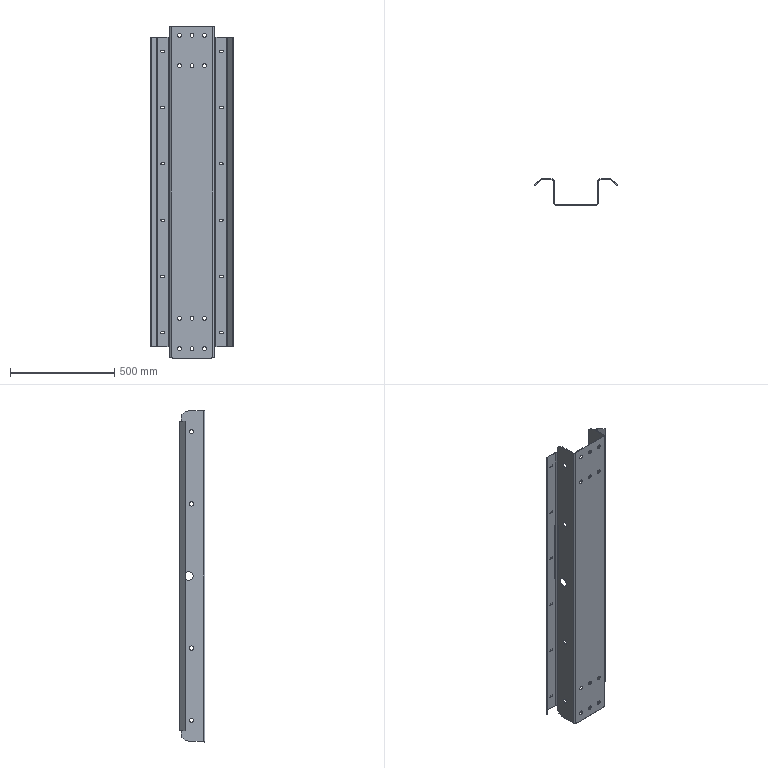Part | STEP file | SYL_0392D6J1SYL0380DJ100-774312 | 1 solid | 162 faces | box 394.569 x 123 x 1592 mm | volume 1976035 mm3 | cylinder 84 | plane 78 | commonest cylinder face diameters 18 x28 10 x26 21 x16 22 x4 41 x4 100 x4